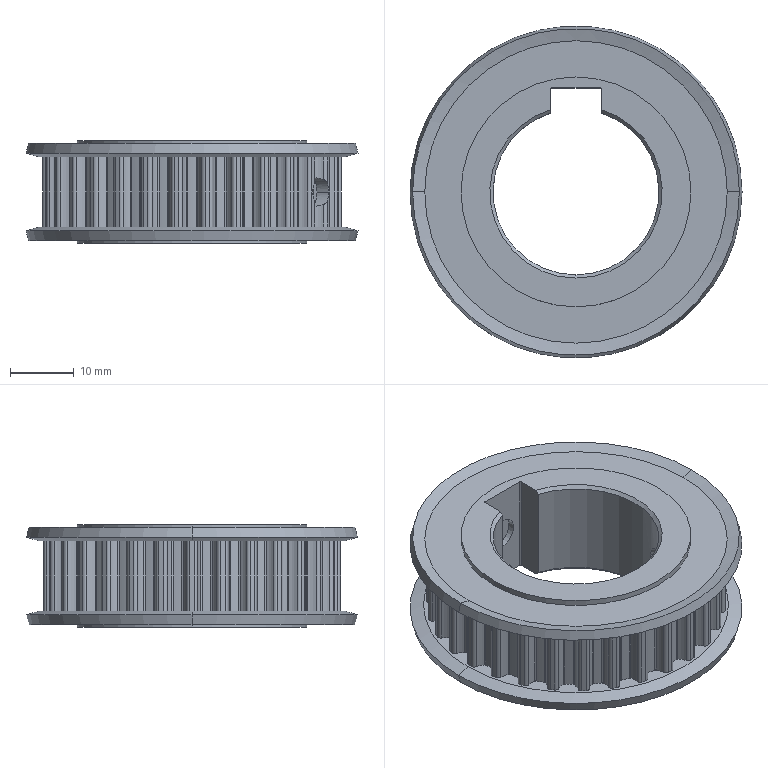Part | SolidWorks | features BaseBody 1 | 1 solid | 312 faces | box 52 x 52 x 16 mm | volume 16805 mm3 | cylinder 269 | plane 27 | cone 16 | commonest cylinder face diameters 0.5 x64 1.1 x64 6.55 x64 43.25 x32 46.79 x30 4.917 x8